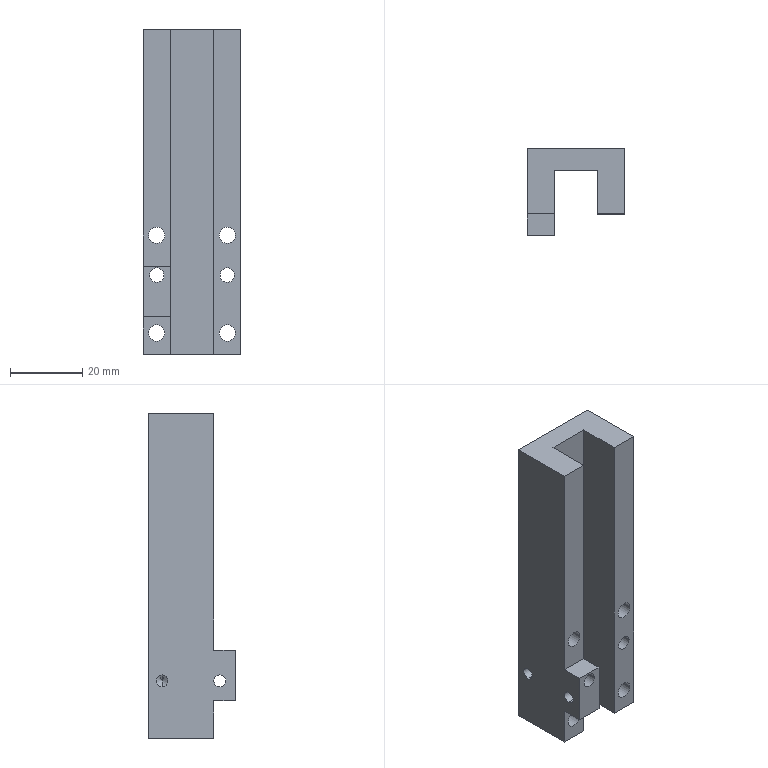Part | NX | features BREP 1 | 1 solid | 32 faces | box 27 x 24 x 90 mm | volume 29584 mm3 | cylinder 16 | plane 14 | cone 2 | commonest cylinder face diameters 4.5 x8 3.3 x4 4 x4
STEP:
#1=CARTESIAN_POINT('',(-774.389,-16.544,14.35));
#2=VERTEX_POINT('',#1);
#3=CARTESIAN_POINT('',(-774.389,-16.544,17.65));
#4=VERTEX_POINT('',#3);
#5=CARTESIAN_POINT('',(-774.389,-16.544,16.));
#6=DIRECTION('',(-1.,0.,0.));
#7=DIRECTION('',(0.,-1.,0.));
#8=AXIS2_PLACEMENT_3D('',#5,#6,#7);
#9=CIRCLE('',#8,1.65);
#10=EDGE_CURVE('',#2,#4,#9,.T.);
#11=ORIENTED_EDGE('',*,*,#10,.F.);
#12=CARTESIAN_POINT('',(-781.889,-16.544,14.35));
#13=VERTEX_POINT('',#12);
#14=CARTESIAN_POINT('',(-781.889,-16.544,14.35));
#15=DIRECTION('',(-1.,0.,0.));
#16=VECTOR('',#15,1000.);
#17=LINE('',#14,#16);
#18=EDGE_CURVE('',#13,#2,#17,.F.);
#19=ORIENTED_EDGE('',*,*,#18,.F.);
#20=CARTESIAN_POINT('',(-781.889,-16.544,17.65));
#21=VERTEX_POINT('',#20);
#22=CARTESIAN_POINT('',(-781.889,-16.544,16.));
#23=DIRECTION('',(-1.,0.,0.));
#24=DIRECTION('',(0.,0.,1.));
#25=AXIS2_PLACEMENT_3D('',#22,#23,#24);
#26=CIRCLE('',#25,1.65);
#27=EDGE_CURVE('',#13,#21,#26,.T.);
#28=ORIENTED_EDGE('',*,*,#27,.T.);
#29=CARTESIAN_POINT('',(-781.889,-16.544,17.65));
#30=DIRECTION('',(-1.,0.,0.));
#31=VECTOR('',#30,1000.);
#32=LINE('',#29,#31);
#33=EDGE_CURVE('',#21,#4,#32,.F.);
#34=ORIENTED_EDGE('',*,*,#33,.T.);
#35=EDGE_LOOP('',(#11,#19,#28,#34));
#36=FACE_BOUND('',#35,.T.);
#37=CARTESIAN_POINT('',(-781.889,-16.544,16.));
#38=DIRECTION('',(-1.,0.,0.));
#39=DIRECTION('',(0.,0.,1.));
#40=AXIS2_PLACEMENT_3D('',#37,#38,#39);
#41=CYLINDRICAL_SURFACE('',#40,1.65);
#42=ADVANCED_FACE('',(#36),#41,.F.);
#43=CARTESIAN_POINT('',(-771.789,-0.5442,14.35));
#44=VERTEX_POINT('',#43);
#45=CARTESIAN_POINT('',(-771.789,-0.5442,17.65));
#46=VERTEX_POINT('',#45);
#47=CARTESIAN_POINT('',(-771.789,-0.5442,16.));
#48=DIRECTION('',(-1.,0.,0.));
#49=DIRECTION('',(0.,0.,1.));
#50=AXIS2_PLACEMENT_3D('',#47,#48,#49);
#51=CIRCLE('',#50,1.65);
#52=EDGE_CURVE('',#44,#46,#51,.T.);
#53=ORIENTED_EDGE('',*,*,#52,.F.);
#54=CARTESIAN_POINT('',(-781.889,-0.5442,14.35));
#55=VERTEX_POINT('',#54);
#56=CARTESIAN_POINT('',(-781.889,-0.5442,14.35));
#57=DIRECTION('',(-1.,0.,0.));
#58=VECTOR('',#57,1000.);
#59=LINE('',#56,#58);
#60=EDGE_CURVE('',#55,#44,#59,.F.);
#61=ORIENTED_EDGE('',*,*,#60,.F.);
#62=CARTESIAN_POINT('',(-781.889,-0.5442,17.65));
#63=VERTEX_POINT('',#62);
#64=CARTESIAN_POINT('',(-781.889,-0.5442,16.));
#65=DIRECTION('',(-1.,0.,0.));
#66=DIRECTION('',(0.,0.,1.));
#67=AXIS2_PLACEMENT_3D('',#64,#65,#66);
#68=CIRCLE('',#67,1.65);
#69=EDGE_CURVE('',#55,#63,#68,.T.);
#70=ORIENTED_EDGE('',*,*,#69,.T.);
#71=CARTESIAN_POINT('',(-781.889,-0.5442,17.65));
#72=DIRECTION('',(-1.,0.,0.));
#73=VECTOR('',#72,1000.);
#74=LINE('',#71,#73);
#75=EDGE_CURVE('',#63,#46,#74,.F.);
#76=ORIENTED_EDGE('',*,*,#75,.T.);
#77=EDGE_LOOP('',(#53,#61,#70,#76));
#78=FACE_BOUND('',#77,.T.);
#79=CARTESIAN_POINT('',(-781.889,-0.5442,16.));
#80=DIRECTION('',(-1.,0.,0.));
#81=DIRECTION('',(0.,0.,1.));
#82=AXIS2_PLACEMENT_3D('',#79,#80,#81);
#83=CYLINDRICAL_SURFACE('',#82,1.65);
#84=ADVANCED_FACE('',(#78),#83,.F.);
#85=CARTESIAN_POINT('',(-770.797,-0.5442,16.));
#86=VERTEX_POINT('',#85);
#87=CARTESIAN_POINT('',(-771.789,-0.5442,17.65));
#88=DIRECTION('',(-0.515,0.,0.8572));
#89=VECTOR('',#88,1000.);
#90=LINE('',#87,#89);
#91=EDGE_CURVE('',#46,#86,#90,.F.);
#92=ORIENTED_EDGE('',*,*,#91,.T.);
#93=CARTESIAN_POINT('',(-771.789,-0.5442,14.35));
#94=DIRECTION('',(-0.515,0.,-0.8572));
#95=VECTOR('',#94,1000.);
#96=LINE('',#93,#95);
#97=EDGE_CURVE('',#44,#86,#96,.F.);
#98=ORIENTED_EDGE('',*,*,#97,.F.);
#99=ORIENTED_EDGE('',*,*,#52,.T.);
#100=EDGE_LOOP('',(#92,#98,#99));
#101=FACE_BOUND('',#100,.T.);
#102=CARTESIAN_POINT('',(-771.789,-0.5442,16.));
#103=DIRECTION('',(-1.,0.,0.));
#104=DIRECTION('',(0.,0.,1.));
#105=AXIS2_PLACEMENT_3D('',#102,#103,#104);
#106=CONICAL_SURFACE('',#105,1.65,1.03);
#107=ADVANCED_FACE('',(#101),#106,.F.);
#108=CARTESIAN_POINT('',(-780.389,3.168,33.));
#109=VERTEX_POINT('',#108);
#110=CARTESIAN_POINT('',(-775.889,3.168,33.));
#111=VERTEX_POINT('',#110);
#112=CARTESIAN_POINT('',(-778.139,3.168,33.));
#113=DIRECTION('',(0.,-1.,0.));
#114=DIRECTION('',(-1.,0.,0.));
#115=AXIS2_PLACEMENT_3D('',#112,#113,#114);
#116=CIRCLE('',#115,2.25);
#117=EDGE_CURVE('',#109,#111,#116,.T.);
#118=ORIENTED_EDGE('',*,*,#117,.F.);
#119=CARTESIAN_POINT('',(-780.389,-14.832,33.));
#120=VERTEX_POINT('',#119);
#121=CARTESIAN_POINT('',(-780.389,3.168,33.));
#122=DIRECTION('',(0.,-1.,0.));
#123=VECTOR('',#122,1000.);
#124=LINE('',#121,#123);
#125=EDGE_CURVE('',#120,#109,#124,.F.);
#126=ORIENTED_EDGE('',*,*,#125,.F.);
#127=CARTESIAN_POINT('',(-775.889,-14.832,33.));
#128=VERTEX_POINT('',#127);
#129=CARTESIAN_POINT('',(-778.139,-14.832,33.));
#130=DIRECTION('',(0.,-1.,0.));
#131=DIRECTION('',(-1.,0.,0.));
#132=AXIS2_PLACEMENT_3D('',#129,#130,#131);
#133=CIRCLE('',#132,2.25);
#134=EDGE_CURVE('',#120,#128,#133,.T.);
#135=ORIENTED_EDGE('',*,*,#134,.T.);
#136=CARTESIAN_POINT('',(-775.889,3.168,33.));
#137=DIRECTION('',(0.,-1.,0.));
#138=VECTOR('',#137,1000.);
#139=LINE('',#136,#138);
#140=EDGE_CURVE('',#128,#111,#139,.F.);
#141=ORIENTED_EDGE('',*,*,#140,.T.);
#142=EDGE_LOOP('',(#118,#126,#135,#141));
#143=FACE_BOUND('',#142,.T.);
#144=CARTESIAN_POINT('',(-778.139,3.168,33.));
#145=DIRECTION('',(0.,-1.,0.));
#146=DIRECTION('',(1.,0.,0.));
#147=AXIS2_PLACEMENT_3D('',#144,#145,#146);
#148=CYLINDRICAL_SURFACE('',#147,2.25);
#149=ADVANCED_FACE('',(#143),#148,.F.);
#150=CARTESIAN_POINT('',(-780.389,3.168,6.));
#151=VERTEX_POINT('',#150);
#152=CARTESIAN_POINT('',(-775.889,3.168,6.));
#153=VERTEX_POINT('',#152);
#154=CARTESIAN_POINT('',(-778.139,3.168,6.));
#155=DIRECTION('',(0.,-1.,0.));
#156=DIRECTION('',(-1.,0.,0.));
#157=AXIS2_PLACEMENT_3D('',#154,#155,#156);
#158=CIRCLE('',#157,2.25);
#159=EDGE_CURVE('',#151,#153,#158,.T.);
#160=ORIENTED_EDGE('',*,*,#159,.F.);
#161=CARTESIAN_POINT('',(-780.389,-14.832,6.));
#162=VERTEX_POINT('',#161);
#163=CARTESIAN_POINT('',(-780.389,3.168,6.));
#164=DIRECTION('',(0.,-1.,0.));
#165=VECTOR('',#164,1000.);
#166=LINE('',#163,#165);
#167=EDGE_CURVE('',#162,#151,#166,.F.);
#168=ORIENTED_EDGE('',*,*,#167,.F.);
#169=CARTESIAN_POINT('',(-775.889,-14.832,6.));
#170=VERTEX_POINT('',#169);
#171=CARTESIAN_POINT('',(-778.139,-14.832,6.));
#172=DIRECTION('',(0.,-1.,0.));
#173=DIRECTION('',(-1.,0.,0.));
#174=AXIS2_PLACEMENT_3D('',#171,#172,#173);
#175=CIRCLE('',#174,2.25);
#176=EDGE_CURVE('',#162,#170,#175,.T.);
#177=ORIENTED_EDGE('',*,*,#176,.T.);
#178=CARTESIAN_POINT('',(-775.889,3.168,6.));
#179=DIRECTION('',(0.,-1.,0.));
#180=VECTOR('',#179,1000.);
#181=LINE('',#178,#180);
#182=EDGE_CURVE('',#170,#153,#181,.F.);
#183=ORIENTED_EDGE('',*,*,#182,.T.);
#184=EDGE_LOOP('',(#160,#168,#177,#183));
#185=FACE_BOUND('',#184,.T.);
#186=CARTESIAN_POINT('',(-778.139,3.168,6.));
#187=DIRECTION('',(0.,-1.,0.));
#188=DIRECTION('',(1.,0.,0.));
#189=AXIS2_PLACEMENT_3D('',#186,#187,#188);
#190=CYLINDRICAL_SURFACE('',#189,2.25);
#191=ADVANCED_FACE('',(#185),#190,.F.);
#192=CARTESIAN_POINT('',(-780.139,3.168,22.));
#193=VERTEX_POINT('',#192);
#194=CARTESIAN_POINT('',(-776.139,3.168,22.));
#195=VERTEX_POINT('',#194);
#196=CARTESIAN_POINT('',(-778.139,3.168,22.));
#197=DIRECTION('',(0.,-1.,0.));
#198=DIRECTION('',(-1.,0.,0.));
#199=AXIS2_PLACEMENT_3D('',#196,#197,#198);
#200=CIRCLE('',#199,2.);
#201=EDGE_CURVE('',#193,#195,#200,.T.);
#202=ORIENTED_EDGE('',*,*,#201,.F.);
#203=CARTESIAN_POINT('',(-780.139,-20.832,22.));
#204=VERTEX_POINT('',#203);
#205=CARTESIAN_POINT('',(-780.139,3.168,22.));
#206=DIRECTION('',(0.,-1.,0.));
#207=VECTOR('',#206,1000.);
#208=LINE('',#205,#207);
#209=EDGE_CURVE('',#204,#193,#208,.F.);
#210=ORIENTED_EDGE('',*,*,#209,.F.);
#211=CARTESIAN_POINT('',(-776.139,-20.832,22.));
#212=VERTEX_POINT('',#211);
#213=CARTESIAN_POINT('',(-778.139,-20.832,22.));
#214=DIRECTION('',(0.,-1.,0.));
#215=DIRECTION('',(1.,0.,0.));
#216=AXIS2_PLACEMENT_3D('',#213,#214,#215);
#217=CIRCLE('',#216,2.);
#218=EDGE_CURVE('',#204,#212,#217,.T.);
#219=ORIENTED_EDGE('',*,*,#218,.T.);
#220=CARTESIAN_POINT('',(-776.139,3.168,22.));
#221=DIRECTION('',(0.,-1.,0.));
#222=VECTOR('',#221,1000.);
#223=LINE('',#220,#222);
#224=EDGE_CURVE('',#212,#195,#223,.F.);
#225=ORIENTED_EDGE('',*,*,#224,.T.);
#226=EDGE_LOOP('',(#202,#210,#219,#225));
#227=FACE_BOUND('',#226,.T.);
#228=CARTESIAN_POINT('',(-778.139,3.168,22.));
#229=DIRECTION('',(0.,-1.,0.));
#230=DIRECTION('',(1.,0.,0.));
#231=AXIS2_PLACEMENT_3D('',#228,#229,#230);
#232=CYLINDRICAL_SURFACE('',#231,2.);
#233=ADVANCED_FACE('',(#227),#232,.F.);
#234=CARTESIAN_POINT('',(-760.639,3.168,22.));
#235=VERTEX_POINT('',#234);
#236=CARTESIAN_POINT('',(-756.639,3.168,22.));
#237=VERTEX_POINT('',#236);
#238=CARTESIAN_POINT('',(-758.639,3.168,22.));
#239=DIRECTION('',(0.,-1.,0.));
#240=DIRECTION('',(1.,0.,0.));
#241=AXIS2_PLACEMENT_3D('',#238,#239,#240);
#242=CIRCLE('',#241,2.);
#243=EDGE_CURVE('',#235,#237,#242,.T.);
#244=ORIENTED_EDGE('',*,*,#243,.F.);
#245=CARTESIAN_POINT('',(-760.639,-14.832,22.));
#246=VERTEX_POINT('',#245);
#247=CARTESIAN_POINT('',(-760.639,3.168,22.));
#248=DIRECTION('',(0.,-1.,0.));
#249=VECTOR('',#248,1000.);
#250=LINE('',#247,#249);
#251=EDGE_CURVE('',#246,#235,#250,.F.);
#252=ORIENTED_EDGE('',*,*,#251,.F.);
#253=CARTESIAN_POINT('',(-756.639,-14.832,22.));
#254=VERTEX_POINT('',#253);
#255=CARTESIAN_POINT('',(-758.639,-14.832,22.));
#256=DIRECTION('',(0.,-1.,0.));
#257=DIRECTION('',(1.,0.,0.));
#258=AXIS2_PLACEMENT_3D('',#255,#256,#257);
#259=CIRCLE('',#258,2.);
#260=EDGE_CURVE('',#246,#254,#259,.T.);
#261=ORIENTED_EDGE('',*,*,#260,.T.);
#262=CARTESIAN_POINT('',(-756.639,3.168,22.));
#263=DIRECTION('',(0.,-1.,0.));
#264=VECTOR('',#263,1000.);
#265=LINE('',#262,#264);
#266=EDGE_CURVE('',#254,#237,#265,.F.);
#267=ORIENTED_EDGE('',*,*,#266,.T.);
#268=EDGE_LOOP('',(#244,#252,#261,#267));
#269=FACE_BOUND('',#268,.T.);
#270=CARTESIAN_POINT('',(-758.639,3.168,22.));
#271=DIRECTION('',(0.,-1.,0.));
#272=DIRECTION('',(1.,0.,0.));
#273=AXIS2_PLACEMENT_3D('',#270,#271,#272);
#274=CYLINDRICAL_SURFACE('',#273,2.);
#275=ADVANCED_FACE('',(#269),#274,.F.);
#276=CARTESIAN_POINT('',(-760.889,3.168,6.));
#277=VERTEX_POINT('',#276);
#278=CARTESIAN_POINT('',(-756.389,3.168,6.));
#279=VERTEX_POINT('',#278);
#280=CARTESIAN_POINT('',(-758.639,3.168,6.));
#281=DIRECTION('',(0.,-1.,0.));
#282=DIRECTION('',(1.,0.,0.));
#283=AXIS2_PLACEMENT_3D('',#280,#281,#282);
#284=CIRCLE('',#283,2.25);
#285=EDGE_CURVE('',#277,#279,#284,.T.);
#286=ORIENTED_EDGE('',*,*,#285,.F.);
#287=CARTESIAN_POINT('',(-760.889,-14.832,6.));
#288=VERTEX_POINT('',#287);
#289=CARTESIAN_POINT('',(-760.889,3.168,6.));
#290=DIRECTION('',(0.,-1.,0.));
#291=VECTOR('',#290,1000.);
#292=LINE('',#289,#291);
#293=EDGE_CURVE('',#288,#277,#292,.F.);
#294=ORIENTED_EDGE('',*,*,#293,.F.);
#295=CARTESIAN_POINT('',(-756.389,-14.832,6.));
#296=VERTEX_POINT('',#295);
#297=CARTESIAN_POINT('',(-758.639,-14.832,6.));
#298=DIRECTION('',(0.,-1.,0.));
#299=DIRECTION('',(1.,0.,0.));
#300=AXIS2_PLACEMENT_3D('',#297,#298,#299);
#301=CIRCLE('',#300,2.25);
#302=EDGE_CURVE('',#288,#296,#301,.T.);
#303=ORIENTED_EDGE('',*,*,#302,.T.);
#304=CARTESIAN_POINT('',(-756.389,3.168,6.));
#305=DIRECTION('',(0.,-1.,0.));
#306=VECTOR('',#305,1000.);
#307=LINE('',#304,#306);
#308=EDGE_CURVE('',#296,#279,#307,.F.);
#309=ORIENTED_EDGE('',*,*,#308,.T.);
#310=EDGE_LOOP('',(#286,#294,#303,#309));
#311=FACE_BOUND('',#310,.T.);
#312=CARTESIAN_POINT('',(-758.639,3.168,6.));
#313=DIRECTION('',(0.,-1.,0.));
#314=DIRECTION('',(1.,0.,0.));
#315=AXIS2_PLACEMENT_3D('',#312,#313,#314);
#316=CYLINDRICAL_SURFACE('',#315,2.25);
#317=ADVANCED_FACE('',(#311),#316,.F.);
#318=CARTESIAN_POINT('',(-760.889,3.168,33.));
#319=VERTEX_POINT('',#318);
#320=CARTESIAN_POINT('',(-756.389,3.168,33.));
#321=VERTEX_POINT('',#320);
#322=CARTESIAN_POINT('',(-758.639,3.168,33.));
#323=DIRECTION('',(0.,-1.,0.));
#324=DIRECTION('',(1.,0.,0.));
#325=AXIS2_PLACEMENT_3D('',#322,#323,#324);
#326=CIRCLE('',#325,2.25);
#327=EDGE_CURVE('',#319,#321,#326,.T.);
#328=ORIENTED_EDGE('',*,*,#327,.F.);
#329=CARTESIAN_POINT('',(-760.889,-14.832,33.));
#330=VERTEX_POINT('',#329);
#331=CARTESIAN_POINT('',(-760.889,3.168,33.));
#332=DIRECTION('',(0.,-1.,0.));
#333=VECTOR('',#332,1000.);
#334=LINE('',#331,#333);
#335=EDGE_CURVE('',#330,#319,#334,.F.);
#336=ORIENTED_EDGE('',*,*,#335,.F.);
#337=CARTESIAN_POINT('',(-756.389,-14.832,33.));
#338=VERTEX_POINT('',#337);
#339=CARTESIAN_POINT('',(-758.639,-14.832,33.));
#340=DIRECTION('',(0.,-1.,0.));
#341=DIRECTION('',(1.,0.,0.));
#342=AXIS2_PLACEMENT_3D('',#339,#340,#341);
#343=CIRCLE('',#342,2.25);
#344=EDGE_CURVE('',#330,#338,#343,.T.);
#345=ORIENTED_EDGE('',*,*,#344,.T.);
#346=CARTESIAN_POINT('',(-756.389,3.168,33.));
#347=DIRECTION('',(0.,-1.,0.));
#348=VECTOR('',#347,1000.);
#349=LINE('',#346,#348);
#350=EDGE_CURVE('',#338,#321,#349,.F.);
#351=ORIENTED_EDGE('',*,*,#350,.T.);
#352=EDGE_LOOP('',(#328,#336,#345,#351));
#353=FACE_BOUND('',#352,.T.);
#354=CARTESIAN_POINT('',(-758.639,3.168,33.));
#355=DIRECTION('',(0.,-1.,0.));
#356=DIRECTION('',(1.,0.,0.));
#357=AXIS2_PLACEMENT_3D('',#354,#355,#356);
#358=CYLINDRICAL_SURFACE('',#357,2.25);
#359=ADVANCED_FACE('',(#353),#358,.F.);
#360=CARTESIAN_POINT('',(-774.389,-14.832,24.5));
#361=VERTEX_POINT('',#360);
#362=CARTESIAN_POINT('',(-781.889,-14.832,24.5));
#363=VERTEX_POINT('',#362);
#364=CARTESIAN_POINT('',(-774.389,-14.832,24.5));
#365=DIRECTION('',(-1.,0.,0.));
#366=VECTOR('',#365,1000.);
#367=LINE('',#364,#366);
#368=EDGE_CURVE('',#361,#363,#367,.T.);
#369=ORIENTED_EDGE('',*,*,#368,.F.);
#370=CARTESIAN_POINT('',(-774.389,-14.832,90.));
#371=VERTEX_POINT('',#370);
#372=CARTESIAN_POINT('',(-774.389,-14.832,0.));
#373=DIRECTION('',(0.,0.,1.));
#374=VECTOR('',#373,1000.);
#375=LINE('',#372,#374);
#376=EDGE_CURVE('',#361,#371,#375,.T.);
#377=ORIENTED_EDGE('',*,*,#376,.T.);
#378=CARTESIAN_POINT('',(-781.889,-14.832,90.));
#379=VERTEX_POINT('',#378);
#380=CARTESIAN_POINT('',(-754.889,-14.832,90.));
#381=DIRECTION('',(1.,0.,0.));
#382=VECTOR('',#381,1000.);
#383=LINE('',#380,#382);
#384=EDGE_CURVE('',#379,#371,#383,.T.);
#385=ORIENTED_EDGE('',*,*,#384,.F.);
#386=CARTESIAN_POINT('',(-781.889,-14.832,90.));
#387=DIRECTION('',(0.,0.,-1.));
#388=VECTOR('',#387,1000.);
#389=LINE('',#386,#388);
#390=EDGE_CURVE('',#379,#363,#389,.T.);
#391=ORIENTED_EDGE('',*,*,#390,.T.);
#392=EDGE_LOOP('',(#369,#377,#385,#391));
#393=FACE_BOUND('',#392,.T.);
#394=CARTESIAN_POINT('',(-778.139,-14.832,33.));
#395=DIRECTION('',(0.,-1.,0.));
#396=DIRECTION('',(-1.,0.,0.));
#397=AXIS2_PLACEMENT_3D('',#394,#395,#396);
#398=CIRCLE('',#397,2.25);
#399=EDGE_CURVE('',#128,#120,#398,.T.);
#400=ORIENTED_EDGE('',*,*,#399,.F.);
#401=ORIENTED_EDGE('',*,*,#134,.F.);
#402=EDGE_LOOP('',(#400,#401));
#403=FACE_BOUND('',#402,.T.);
#404=CARTESIAN_POINT('',(-754.889,-14.832,90.));
#405=DIRECTION('',(0.,1.,0.));
#406=DIRECTION('',(1.,0.,0.));
#407=AXIS2_PLACEMENT_3D('',#404,#405,#406);
#408=PLANE('',#407);
#409=ADVANCED_FACE('',(#393,#403),#408,.F.);
#410=CARTESIAN_POINT('',(-781.889,-14.832,10.5));
#411=VERTEX_POINT('',#410);
#412=CARTESIAN_POINT('',(-774.389,-14.832,10.5));
#413=VERTEX_POINT('',#412);
#414=CARTESIAN_POINT('',(-774.389,-14.832,10.5));
#415=DIRECTION('',(1.,0.,0.));
#416=VECTOR('',#415,1000.);
#417=LINE('',#414,#416);
#418=EDGE_CURVE('',#411,#413,#417,.T.);
#419=ORIENTED_EDGE('',*,*,#418,.F.);
#420=CARTESIAN_POINT('',(-781.889,-14.832,0.));
#421=VERTEX_POINT('',#420);
#422=CARTESIAN_POINT('',(-781.889,-14.832,90.));
#423=DIRECTION('',(0.,0.,-1.));
#424=VECTOR('',#423,1000.);
#425=LINE('',#422,#424);
#426=EDGE_CURVE('',#411,#421,#425,.T.);
#427=ORIENTED_EDGE('',*,*,#426,.T.);
#428=CARTESIAN_POINT('',(-774.389,-14.832,0.));
#429=VERTEX_POINT('',#428);
#430=CARTESIAN_POINT('',(-754.889,-14.832,0.));
#431=DIRECTION('',(1.,0.,0.));
#432=VECTOR('',#431,1000.);
#433=LINE('',#430,#432);
#434=EDGE_CURVE('',#421,#429,#433,.T.);
#435=ORIENTED_EDGE('',*,*,#434,.T.);
#436=CARTESIAN_POINT('',(-774.389,-14.832,0.));
#437=DIRECTION('',(0.,0.,1.));
#438=VECTOR('',#437,1000.);
#439=LINE('',#436,#438);
#440=EDGE_CURVE('',#429,#413,#439,.T.);
#441=ORIENTED_EDGE('',*,*,#440,.T.);
#442=EDGE_LOOP('',(#419,#427,#435,#441));
#443=FACE_BOUND('',#442,.T.);
#444=CARTESIAN_POINT('',(-778.139,-14.832,6.));
#445=DIRECTION('',(0.,-1.,0.));
#446=DIRECTION('',(-1.,0.,0.));
#447=AXIS2_PLACEMENT_3D('',#444,#445,#446);
#448=CIRCLE('',#447,2.25);
#449=EDGE_CURVE('',#170,#162,#448,.T.);
#450=ORIENTED_EDGE('',*,*,#449,.F.);
#451=ORIENTED_EDGE('',*,*,#176,.F.);
#452=EDGE_LOOP('',(#450,#451));
#453=FACE_BOUND('',#452,.T.);
#454=CARTESIAN_POINT('',(-754.889,-14.832,90.));
#455=DIRECTION('',(0.,1.,0.));
#456=DIRECTION('',(1.,0.,0.));
#457=AXIS2_PLACEMENT_3D('',#454,#455,#456);
#458=PLANE('',#457);
#459=ADVANCED_FACE('',(#443,#453),#458,.F.);
#460=CARTESIAN_POINT('',(-762.389,-14.832,90.));
#461=VERTEX_POINT('',#460);
#462=CARTESIAN_POINT('',(-754.889,-14.832,90.));
#463=VERTEX_POINT('',#462);
#464=CARTESIAN_POINT('',(-754.889,-14.832,90.));
#465=DIRECTION('',(1.,0.,0.));
#466=VECTOR('',#465,1000.);
#467=LINE('',#464,#466);
#468=EDGE_CURVE('',#461,#463,#467,.T.);
#469=ORIENTED_EDGE('',*,*,#468,.F.);
#470=CARTESIAN_POINT('',(-762.389,-14.832,0.));
#471=VERTEX_POINT('',#470);
#472=CARTESIAN_POINT('',(-762.389,-14.832,0.));
#473=DIRECTION('',(0.,0.,1.));
#474=VECTOR('',#473,1000.);
#475=LINE('',#472,#474);
#476=EDGE_CURVE('',#471,#461,#475,.T.);
#477=ORIENTED_EDGE('',*,*,#476,.F.);
#478=CARTESIAN_POINT('',(-754.889,-14.832,0.));
#479=VERTEX_POINT('',#478);
#480=CARTESIAN_POINT('',(-754.889,-14.832,0.));
#481=DIRECTION('',(1.,0.,0.));
#482=VECTOR('',#481,1000.);
#483=LINE('',#480,#482);
#484=EDGE_CURVE('',#471,#479,#483,.T.);
#485=ORIENTED_EDGE('',*,*,#484,.T.);
#486=CARTESIAN_POINT('',(-754.889,-14.832,90.));
#487=DIRECTION('',(0.,0.,-1.));
#488=VECTOR('',#487,1000.);
#489=LINE('',#486,#488);
#490=EDGE_CURVE('',#463,#479,#489,.T.);
#491=ORIENTED_EDGE('',*,*,#490,.F.);
#492=EDGE_LOOP('',(#469,#477,#485,#491));
#493=FACE_BOUND('',#492,.T.);
#494=CARTESIAN_POINT('',(-758.639,-14.832,22.));
#495=DIRECTION('',(0.,-1.,0.));
#496=DIRECTION('',(1.,0.,0.));
#497=AXIS2_PLACEMENT_3D('',#494,#495,#496);
#498=CIRCLE('',#497,2.);
#499=EDGE_CURVE('',#254,#246,#498,.T.);
#500=ORIENTED_EDGE('',*,*,#499,.F.);
#501=ORIENTED_EDGE('',*,*,#260,.F.);
#502=EDGE_LOOP('',(#500,#501));
#503=FACE_BOUND('',#502,.T.);
#504=CARTESIAN_POINT('',(-758.639,-14.832,6.));
#505=DIRECTION('',(0.,-1.,0.));
#506=DIRECTION('',(1.,0.,0.));
#507=AXIS2_PLACEMENT_3D('',#504,#505,#506);
#508=CIRCLE('',#507,2.25);
#509=EDGE_CURVE('',#296,#288,#508,.T.);
#510=ORIENTED_EDGE('',*,*,#509,.F.);
#511=ORIENTED_EDGE('',*,*,#302,.F.);
#512=EDGE_LOOP('',(#510,#511));
#513=FACE_BOUND('',#512,.T.);
#514=CARTESIAN_POINT('',(-758.639,-14.832,33.));
#515=DIRECTION('',(0.,-1.,0.));
#516=DIRECTION('',(1.,0.,0.));
#517=AXIS2_PLACEMENT_3D('',#514,#515,#516);
#518=CIRCLE('',#517,2.25);
#519=EDGE_CURVE('',#338,#330,#518,.T.);
#520=ORIENTED_EDGE('',*,*,#519,.F.);
#521=ORIENTED_EDGE('',*,*,#344,.F.);
#522=EDGE_LOOP('',(#520,#521));
#523=FACE_BOUND('',#522,.T.);
#524=CARTESIAN_POINT('',(-754.889,-14.832,90.));
#525=DIRECTION('',(0.,1.,0.));
#526=DIRECTION('',(1.,0.,0.));
#527=AXIS2_PLACEMENT_3D('',#524,#525,#526);
#528=PLANE('',#527);
#529=ADVANCED_FACE('',(#493,#503,#513,#523),#528,.F.);
#530=CARTESIAN_POINT('',(-754.889,3.168,0.));
#531=VERTEX_POINT('',#530);
#532=CARTESIAN_POINT('',(-754.889,-14.832,0.));
#533=DIRECTION('',(0.,1.,0.));
#534=VECTOR('',#533,1000.);
#535=LINE('',#532,#534);
#536=EDGE_CURVE('',#479,#531,#535,.T.);
#537=ORIENTED_EDGE('',*,*,#536,.T.);
#538=CARTESIAN_POINT('',(-754.889,3.168,90.));
#539=VERTEX_POINT('',#538);
#540=CARTESIAN_POINT('',(-754.889,3.168,90.));
#541=DIRECTION('',(0.,0.,-1.));
#542=VECTOR('',#541,1000.);
#543=LINE('',#540,#542);
#544=EDGE_CURVE('',#539,#531,#543,.T.);
#545=ORIENTED_EDGE('',*,*,#544,.F.);
#546=CARTESIAN_POINT('',(-754.889,-14.832,90.));
#547=DIRECTION('',(0.,1.,0.));
#548=VECTOR('',#547,1000.);
#549=LINE('',#546,#548);
#550=EDGE_CURVE('',#463,#539,#549,.T.);
#551=ORIENTED_EDGE('',*,*,#550,.F.);
#552=ORIENTED_EDGE('',*,*,#490,.T.);
#553=EDGE_LOOP('',(#537,#545,#551,#552));
#554=FACE_BOUND('',#553,.T.);
#555=CARTESIAN_POINT('',(-754.889,-14.832,90.));
#556=DIRECTION('',(-1.,0.,0.));
#557=DIRECTION('',(0.,0.,1.));
#558=AXIS2_PLACEMENT_3D('',#555,#556,#557);
#559=PLANE('',#558);
#560=ADVANCED_FACE('',(#554),#559,.F.);
#561=CARTESIAN_POINT('',(-781.889,3.168,0.));
#562=VERTEX_POINT('',#561);
#563=CARTESIAN_POINT('',(-754.889,3.168,0.));
#564=DIRECTION('',(-1.,0.,0.));
#565=VECTOR('',#564,1000.);
#566=LINE('',#563,#565);
#567=EDGE_CURVE('',#531,#562,#566,.T.);
#568=ORIENTED_EDGE('',*,*,#567,.T.);
#569=CARTESIAN_POINT('',(-781.889,3.168,90.));
#570=VERTEX_POINT('',#569);
#571=CARTESIAN_POINT('',(-781.889,3.168,90.));
#572=DIRECTION('',(0.,0.,-1.));
#573=VECTOR('',#572,1000.);
#574=LINE('',#571,#573);
#575=EDGE_CURVE('',#570,#562,#574,.T.);
#576=ORIENTED_EDGE('',*,*,#575,.F.);
#577=CARTESIAN_POINT('',(-754.889,3.168,90.));
#578=DIRECTION('',(-1.,0.,0.));
#579=VECTOR('',#578,1000.);
#580=LINE('',#577,#579);
#581=EDGE_CURVE('',#539,#570,#580,.T.);
#582=ORIENTED_EDGE('',*,*,#581,.F.);
#583=ORIENTED_EDGE('',*,*,#544,.T.);
#584=EDGE_LOOP('',(#568,#576,#582,#583));
#585=FACE_BOUND('',#584,.T.);
#586=CARTESIAN_POINT('',(-778.139,3.168,33.));
#587=DIRECTION('',(0.,-1.,0.));
#588=DIRECTION('',(-1.,0.,0.));
#589=AXIS2_PLACEMENT_3D('',#586,#587,#588);
#590=CIRCLE('',#589,2.25);
#591=EDGE_CURVE('',#111,#109,#590,.T.);
#592=ORIENTED_EDGE('',*,*,#591,.T.);
#593=ORIENTED_EDGE('',*,*,#117,.T.);
#594=EDGE_LOOP('',(#592,#593));
#595=FACE_BOUND('',#594,.T.);
#596=CARTESIAN_POINT('',(-778.139,3.168,6.));
#597=DIRECTION('',(0.,-1.,0.));
#598=DIRECTION('',(-1.,0.,0.));
#599=AXIS2_PLACEMENT_3D('',#596,#597,#598);
#600=CIRCLE('',#599,2.25);
#601=EDGE_CURVE('',#153,#151,#600,.T.);
#602=ORIENTED_EDGE('',*,*,#601,.T.);
#603=ORIENTED_EDGE('',*,*,#159,.T.);
#604=EDGE_LOOP('',(#602,#603));
#605=FACE_BOUND('',#604,.T.);
#606=CARTESIAN_POINT('',(-778.139,3.168,22.));
#607=DIRECTION('',(0.,-1.,0.));
#608=DIRECTION('',(-1.,0.,0.));
#609=AXIS2_PLACEMENT_3D('',#606,#607,#608);
#610=CIRCLE('',#609,2.);
#611=EDGE_CURVE('',#195,#193,#610,.T.);
#612=ORIENTED_EDGE('',*,*,#611,.T.);
#613=ORIENTED_EDGE('',*,*,#201,.T.);
#614=EDGE_LOOP('',(#612,#613));
#615=FACE_BOUND('',#614,.T.);
#616=CARTESIAN_POINT('',(-758.639,3.168,22.));
#617=DIRECTION('',(0.,-1.,0.));
#618=DIRECTION('',(1.,0.,0.));
#619=AXIS2_PLACEMENT_3D('',#616,#617,#618);
#620=CIRCLE('',#619,2.);
#621=EDGE_CURVE('',#237,#235,#620,.T.);
#622=ORIENTED_EDGE('',*,*,#621,.T.);
#623=ORIENTED_EDGE('',*,*,#243,.T.);
#624=EDGE_LOOP('',(#622,#623));
#625=FACE_BOUND('',#624,.T.);
#626=CARTESIAN_POINT('',(-758.639,3.168,6.));
#627=DIRECTION('',(0.,-1.,0.));
#628=DIRECTION('',(1.,0.,0.));
#629=AXIS2_PLACEMENT_3D('',#626,#627,#628);
#630=CIRCLE('',#629,2.25);
#631=EDGE_CURVE('',#279,#277,#630,.T.);
#632=ORIENTED_EDGE('',*,*,#631,.T.);
#633=ORIENTED_EDGE('',*,*,#285,.T.);
#634=EDGE_LOOP('',(#632,#633));
#635=FACE_BOUND('',#634,.T.);
#636=CARTESIAN_POINT('',(-758.639,3.168,33.));
#637=DIRECTION('',(0.,-1.,0.));
#638=DIRECTION('',(1.,0.,0.));
#639=AXIS2_PLACEMENT_3D('',#636,#637,#638);
#640=CIRCLE('',#639,2.25);
#641=EDGE_CURVE('',#321,#319,#640,.T.);
#642=ORIENTED_EDGE('',*,*,#641,.T.);
#643=ORIENTED_EDGE('',*,*,#327,.T.);
#644=EDGE_LOOP('',(#642,#643));
#645=FACE_BOUND('',#644,.T.);
#646=CARTESIAN_POINT('',(-754.889,3.168,90.));
#647=DIRECTION('',(0.,-1.,0.));
#648=DIRECTION('',(0.,0.,-1.));
#649=AXIS2_PLACEMENT_3D('',#646,#647,#648);
#650=PLANE('',#649);
#651=ADVANCED_FACE('',(#585,#595,#605,#615,#625,#635,#645),#650,.F.);
#652=CARTESIAN_POINT('',(-781.889,-14.832,0.));
#653=DIRECTION('',(0.,-1.,0.));
#654=VECTOR('',#653,1000.);
#655=LINE('',#652,#654);
#656=EDGE_CURVE('',#562,#421,#655,.T.);
#657=ORIENTED_EDGE('',*,*,#656,.T.);
#658=ORIENTED_EDGE('',*,*,#426,.F.);
#659=CARTESIAN_POINT('',(-781.889,-20.832,10.5));
#660=VERTEX_POINT('',#659);
#661=CARTESIAN_POINT('',(-781.889,-20.832,10.5));
#662=DIRECTION('',(0.,1.,0.));
#663=VECTOR('',#662,1000.);
#664=LINE('',#661,#663);
#665=EDGE_CURVE('',#660,#411,#664,.T.);
#666=ORIENTED_EDGE('',*,*,#665,.F.);
#667=CARTESIAN_POINT('',(-781.889,-20.832,24.5));
#668=VERTEX_POINT('',#667);
#669=CARTESIAN_POINT('',(-781.889,-20.832,24.5));
#670=DIRECTION('',(0.,0.,-1.));
#671=VECTOR('',#670,1000.);
#672=LINE('',#669,#671);
#673=EDGE_CURVE('',#668,#660,#672,.T.);
#674=ORIENTED_EDGE('',*,*,#673,.F.);
#675=CARTESIAN_POINT('',(-781.889,-20.832,24.5));
#676=DIRECTION('',(0.,1.,0.));
#677=VECTOR('',#676,1000.);
#678=LINE('',#675,#677);
#679=EDGE_CURVE('',#668,#363,#678,.T.);
#680=ORIENTED_EDGE('',*,*,#679,.T.);
#681=ORIENTED_EDGE('',*,*,#390,.F.);
#682=CARTESIAN_POINT('',(-781.889,-14.832,90.));
#683=DIRECTION('',(0.,-1.,0.));
#684=VECTOR('',#683,1000.);
#685=LINE('',#682,#684);
#686=EDGE_CURVE('',#570,#379,#685,.T.);
#687=ORIENTED_EDGE('',*,*,#686,.F.);
#688=ORIENTED_EDGE('',*,*,#575,.T.);
#689=EDGE_LOOP('',(#657,#658,#666,#674,#680,#681,#687,#688));
#690=FACE_BOUND('',#689,.T.);
#691=CARTESIAN_POINT('',(-781.889,-16.544,16.));
#692=DIRECTION('',(-1.,0.,0.));
#693=DIRECTION('',(0.,0.,1.));
#694=AXIS2_PLACEMENT_3D('',#691,#692,#693);
#695=CIRCLE('',#694,1.65);
#696=EDGE_CURVE('',#21,#13,#695,.T.);
#697=ORIENTED_EDGE('',*,*,#696,.F.);
#698=ORIENTED_EDGE('',*,*,#27,.F.);
#699=EDGE_LOOP('',(#697,#698));
#700=FACE_BOUND('',#699,.T.);
#701=CARTESIAN_POINT('',(-781.889,-0.5442,16.));
#702=DIRECTION('',(-1.,0.,0.));
#703=DIRECTION('',(0.,0.,1.));
#704=AXIS2_PLACEMENT_3D('',#701,#702,#703);
#705=CIRCLE('',#704,1.65);
#706=EDGE_CURVE('',#63,#55,#705,.T.);
#707=ORIENTED_EDGE('',*,*,#706,.F.);
#708=ORIENTED_EDGE('',*,*,#69,.F.);
#709=EDGE_LOOP('',(#707,#708));
#710=FACE_BOUND('',#709,.T.);
#711=CARTESIAN_POINT('',(-781.889,-14.832,90.));
#712=DIRECTION('',(1.,0.,0.));
#713=DIRECTION('',(0.,1.,0.));
#714=AXIS2_PLACEMENT_3D('',#711,#712,#713);
#715=PLANE('',#714);
#716=ADVANCED_FACE('',(#690,#700,#710),#715,.F.);
#717=CARTESIAN_POINT('',(-762.389,-2.832,90.));
#718=VERTEX_POINT('',#717);
#719=CARTESIAN_POINT('',(-762.389,-14.832,90.));
#720=DIRECTION('',(0.,1.,0.));
#721=VECTOR('',#720,1000.);
#722=LINE('',#719,#721);
#723=EDGE_CURVE('',#461,#718,#722,.T.);
#724=ORIENTED_EDGE('',*,*,#723,.F.);
#725=ORIENTED_EDGE('',*,*,#468,.T.);
#726=ORIENTED_EDGE('',*,*,#550,.T.);
#727=ORIENTED_EDGE('',*,*,#581,.T.);
#728=ORIENTED_EDGE('',*,*,#686,.T.);
#729=ORIENTED_EDGE('',*,*,#384,.T.);
#730=CARTESIAN_POINT('',(-774.389,-2.832,90.));
#731=VERTEX_POINT('',#730);
#732=CARTESIAN_POINT('',(-774.389,-14.832,90.));
#733=DIRECTION('',(0.,-1.,0.));
#734=VECTOR('',#733,1000.);
#735=LINE('',#732,#734);
#736=EDGE_CURVE('',#731,#371,#735,.T.);
#737=ORIENTED_EDGE('',*,*,#736,.F.);
#738=CARTESIAN_POINT('',(-762.389,-2.832,90.));
#739=DIRECTION('',(-1.,0.,0.));
#740=VECTOR('',#739,1000.);
#741=LINE('',#738,#740);
#742=EDGE_CURVE('',#718,#731,#741,.T.);
#743=ORIENTED_EDGE('',*,*,#742,.F.);
#744=EDGE_LOOP('',(#724,#725,#726,#727,#728,#729,#737,#743));
#745=FACE_BOUND('',#744,.T.);
#746=CARTESIAN_POINT('',(-754.889,3.168,90.));
#747=DIRECTION('',(0.,0.,1.));
#748=DIRECTION('',(1.,0.,0.));
#749=AXIS2_PLACEMENT_3D('',#746,#747,#748);
#750=PLANE('',#749);
#751=ADVANCED_FACE('',(#745),#750,.T.);
#752=ORIENTED_EDGE('',*,*,#484,.F.);
#753=CARTESIAN_POINT('',(-762.389,-2.832,0.));
#754=VERTEX_POINT('',#753);
#755=CARTESIAN_POINT('',(-762.389,-14.832,0.));
#756=DIRECTION('',(0.,1.,0.));
#757=VECTOR('',#756,1000.);
#758=LINE('',#755,#757);
#759=EDGE_CURVE('',#471,#754,#758,.T.);
#760=ORIENTED_EDGE('',*,*,#759,.T.);
#761=CARTESIAN_POINT('',(-774.389,-2.832,0.));
#762=VERTEX_POINT('',#761);
#763=CARTESIAN_POINT('',(-762.389,-2.832,0.));
#764=DIRECTION('',(-1.,0.,0.));
#765=VECTOR('',#764,1000.);
#766=LINE('',#763,#765);
#767=EDGE_CURVE('',#754,#762,#766,.T.);
#768=ORIENTED_EDGE('',*,*,#767,.T.);
#769=CARTESIAN_POINT('',(-774.389,-14.832,0.));
#770=DIRECTION('',(0.,-1.,0.));
#771=VECTOR('',#770,1000.);
#772=LINE('',#769,#771);
#773=EDGE_CURVE('',#762,#429,#772,.T.);
#774=ORIENTED_EDGE('',*,*,#773,.T.);
#775=ORIENTED_EDGE('',*,*,#434,.F.);
#776=ORIENTED_EDGE('',*,*,#656,.F.);
#777=ORIENTED_EDGE('',*,*,#567,.F.);
#778=ORIENTED_EDGE('',*,*,#536,.F.);
#779=EDGE_LOOP('',(#752,#760,#768,#774,#775,#776,#777,#778));
#780=FACE_BOUND('',#779,.T.);
#781=CARTESIAN_POINT('',(-754.889,3.168,0.));
#782=DIRECTION('',(0.,0.,1.));
#783=DIRECTION('',(1.,0.,0.));
#784=AXIS2_PLACEMENT_3D('',#781,#782,#783);
#785=PLANE('',#784);
#786=ADVANCED_FACE('',(#780),#785,.F.);
#787=ORIENTED_EDGE('',*,*,#723,.T.);
#788=CARTESIAN_POINT('',(-762.389,-2.832,0.));
#789=DIRECTION('',(0.,0.,1.));
#790=VECTOR('',#789,1000.);
#791=LINE('',#788,#790);
#792=EDGE_CURVE('',#754,#718,#791,.T.);
#793=ORIENTED_EDGE('',*,*,#792,.F.);
#794=ORIENTED_EDGE('',*,*,#759,.F.);
#795=ORIENTED_EDGE('',*,*,#476,.T.);
#796=EDGE_LOOP('',(#787,#793,#794,#795));
#797=FACE_BOUND('',#796,.T.);
#798=CARTESIAN_POINT('',(-762.389,-14.832,0.));
#799=DIRECTION('',(1.,0.,0.));
#800=DIRECTION('',(0.,1.,0.));
#801=AXIS2_PLACEMENT_3D('',#798,#799,#800);
#802=PLANE('',#801);
#803=ADVANCED_FACE('',(#797),#802,.F.);
#804=ORIENTED_EDGE('',*,*,#736,.T.);
#805=ORIENTED_EDGE('',*,*,#376,.F.);
#806=CARTESIAN_POINT('',(-774.389,-20.832,24.5));
#807=VERTEX_POINT('',#806);
#808=CARTESIAN_POINT('',(-774.389,-20.832,24.5));
#809=DIRECTION('',(0.,1.,0.));
#810=VECTOR('',#809,1000.);
#811=LINE('',#808,#810);
#812=EDGE_CURVE('',#807,#361,#811,.T.);
#813=ORIENTED_EDGE('',*,*,#812,.F.);
#814=CARTESIAN_POINT('',(-774.389,-20.832,10.5));
#815=VERTEX_POINT('',#814);
#816=CARTESIAN_POINT('',(-774.389,-20.832,24.5));
#817=DIRECTION('',(0.,0.,1.));
#818=VECTOR('',#817,1000.);
#819=LINE('',#816,#818);
#820=EDGE_CURVE('',#815,#807,#819,.T.);
#821=ORIENTED_EDGE('',*,*,#820,.F.);
#822=CARTESIAN_POINT('',(-774.389,-20.832,10.5));
#823=DIRECTION('',(0.,1.,0.));
#824=VECTOR('',#823,1000.);
#825=LINE('',#822,#824);
#826=EDGE_CURVE('',#815,#413,#825,.T.);
#827=ORIENTED_EDGE('',*,*,#826,.T.);
#828=ORIENTED_EDGE('',*,*,#440,.F.);
#829=ORIENTED_EDGE('',*,*,#773,.F.);
#830=CARTESIAN_POINT('',(-774.389,-2.832,0.));
#831=DIRECTION('',(0.,0.,1.));
#832=VECTOR('',#831,1000.);
#833=LINE('',#830,#832);
#834=EDGE_CURVE('',#762,#731,#833,.T.);
#835=ORIENTED_EDGE('',*,*,#834,.T.);
#836=EDGE_LOOP('',(#804,#805,#813,#821,#827,#828,#829,#835));
#837=FACE_BOUND('',#836,.T.);
#838=CARTESIAN_POINT('',(-774.389,-16.544,16.));
#839=DIRECTION('',(-1.,0.,0.));
#840=DIRECTION('',(0.,-1.,0.));
#841=AXIS2_PLACEMENT_3D('',#838,#839,#840);
#842=CIRCLE('',#841,1.65);
#843=EDGE_CURVE('',#4,#2,#842,.T.);
#844=ORIENTED_EDGE('',*,*,#843,.T.);
#845=ORIENTED_EDGE('',*,*,#10,.T.);
#846=EDGE_LOOP('',(#844,#845));
#847=FACE_BOUND('',#846,.T.);
#848=CARTESIAN_POINT('',(-774.389,-14.832,0.));
#849=DIRECTION('',(-1.,0.,0.));
#850=DIRECTION('',(0.,1.,0.));
#851=AXIS2_PLACEMENT_3D('',#848,#849,#850);
#852=PLANE('',#851);
#853=ADVANCED_FACE('',(#837,#847),#852,.F.);
#854=ORIENTED_EDGE('',*,*,#742,.T.);
#855=ORIENTED_EDGE('',*,*,#834,.F.);
#856=ORIENTED_EDGE('',*,*,#767,.F.);
#857=ORIENTED_EDGE('',*,*,#792,.T.);
#858=EDGE_LOOP('',(#854,#855,#856,#857));
#859=FACE_BOUND('',#858,.T.);
#860=CARTESIAN_POINT('',(-762.389,-2.832,0.));
#861=DIRECTION('',(0.,1.,0.));
#862=DIRECTION('',(1.,0.,0.));
#863=AXIS2_PLACEMENT_3D('',#860,#861,#862);
#864=PLANE('',#863);
#865=ADVANCED_FACE('',(#859),#864,.F.);
#866=ORIENTED_EDGE('',*,*,#335,.T.);
#867=ORIENTED_EDGE('',*,*,#641,.F.);
#868=ORIENTED_EDGE('',*,*,#350,.F.);
#869=ORIENTED_EDGE('',*,*,#519,.T.);
#870=EDGE_LOOP('',(#866,#867,#868,#869));
#871=FACE_BOUND('',#870,.T.);
#872=CARTESIAN_POINT('',(-758.639,3.168,33.));
#873=DIRECTION('',(0.,-1.,0.));
#874=DIRECTION('',(1.,0.,0.));
#875=AXIS2_PLACEMENT_3D('',#872,#873,#874);
#876=CYLINDRICAL_SURFACE('',#875,2.25);
#877=ADVANCED_FACE('',(#871),#876,.F.);
#878=ORIENTED_EDGE('',*,*,#293,.T.);
#879=ORIENTED_EDGE('',*,*,#631,.F.);
#880=ORIENTED_EDGE('',*,*,#308,.F.);
#881=ORIENTED_EDGE('',*,*,#509,.T.);
#882=EDGE_LOOP('',(#878,#879,#880,#881));
#883=FACE_BOUND('',#882,.T.);
#884=CARTESIAN_POINT('',(-758.639,3.168,6.));
#885=DIRECTION('',(0.,-1.,0.));
#886=DIRECTION('',(1.,0.,0.));
#887=AXIS2_PLACEMENT_3D('',#884,#885,#886);
#888=CYLINDRICAL_SURFACE('',#887,2.25);
#889=ADVANCED_FACE('',(#883),#888,.F.);
#890=ORIENTED_EDGE('',*,*,#251,.T.);
#891=ORIENTED_EDGE('',*,*,#621,.F.);
#892=ORIENTED_EDGE('',*,*,#266,.F.);
#893=ORIENTED_EDGE('',*,*,#499,.T.);
#894=EDGE_LOOP('',(#890,#891,#892,#893));
#895=FACE_BOUND('',#894,.T.);
#896=CARTESIAN_POINT('',(-758.639,3.168,22.));
#897=DIRECTION('',(0.,-1.,0.));
#898=DIRECTION('',(1.,0.,0.));
#899=AXIS2_PLACEMENT_3D('',#896,#897,#898);
#900=CYLINDRICAL_SURFACE('',#899,2.);
#901=ADVANCED_FACE('',(#895),#900,.F.);
#902=ORIENTED_EDGE('',*,*,#209,.T.);
#903=ORIENTED_EDGE('',*,*,#611,.F.);
#904=ORIENTED_EDGE('',*,*,#224,.F.);
#905=CARTESIAN_POINT('',(-778.139,-20.832,22.));
#906=DIRECTION('',(0.,-1.,0.));
#907=DIRECTION('',(1.,0.,0.));
#908=AXIS2_PLACEMENT_3D('',#905,#906,#907);
#909=CIRCLE('',#908,2.);
#910=EDGE_CURVE('',#212,#204,#909,.T.);
#911=ORIENTED_EDGE('',*,*,#910,.T.);
#912=EDGE_LOOP('',(#902,#903,#904,#911));
#913=FACE_BOUND('',#912,.T.);
#914=CARTESIAN_POINT('',(-778.139,3.168,22.));
#915=DIRECTION('',(0.,-1.,0.));
#916=DIRECTION('',(1.,0.,0.));
#917=AXIS2_PLACEMENT_3D('',#914,#915,#916);
#918=CYLINDRICAL_SURFACE('',#917,2.);
#919=ADVANCED_FACE('',(#913),#918,.F.);
#920=ORIENTED_EDGE('',*,*,#167,.T.);
#921=ORIENTED_EDGE('',*,*,#601,.F.);
#922=ORIENTED_EDGE('',*,*,#182,.F.);
#923=ORIENTED_EDGE('',*,*,#449,.T.);
#924=EDGE_LOOP('',(#920,#921,#922,#923));
#925=FACE_BOUND('',#924,.T.);
#926=CARTESIAN_POINT('',(-778.139,3.168,6.));
#927=DIRECTION('',(0.,-1.,0.));
#928=DIRECTION('',(1.,0.,0.));
#929=AXIS2_PLACEMENT_3D('',#926,#927,#928);
#930=CYLINDRICAL_SURFACE('',#929,2.25);
#931=ADVANCED_FACE('',(#925),#930,.F.);
#932=ORIENTED_EDGE('',*,*,#125,.T.);
#933=ORIENTED_EDGE('',*,*,#591,.F.);
#934=ORIENTED_EDGE('',*,*,#140,.F.);
#935=ORIENTED_EDGE('',*,*,#399,.T.);
#936=EDGE_LOOP('',(#932,#933,#934,#935));
#937=FACE_BOUND('',#936,.T.);
#938=CARTESIAN_POINT('',(-778.139,3.168,33.));
#939=DIRECTION('',(0.,-1.,0.));
#940=DIRECTION('',(1.,0.,0.));
#941=AXIS2_PLACEMENT_3D('',#938,#939,#940);
#942=CYLINDRICAL_SURFACE('',#941,2.25);
#943=ADVANCED_FACE('',(#937),#942,.F.);
#944=ORIENTED_EDGE('',*,*,#820,.T.);
#945=CARTESIAN_POINT('',(-774.389,-20.832,24.5));
#946=DIRECTION('',(-1.,0.,0.));
#947=VECTOR('',#946,1000.);
#948=LINE('',#945,#947);
#949=EDGE_CURVE('',#807,#668,#948,.T.);
#950=ORIENTED_EDGE('',*,*,#949,.T.);
#951=ORIENTED_EDGE('',*,*,#673,.T.);
#952=CARTESIAN_POINT('',(-774.389,-20.832,10.5));
#953=DIRECTION('',(1.,0.,0.));
#954=VECTOR('',#953,1000.);
#955=LINE('',#952,#954);
#956=EDGE_CURVE('',#660,#815,#955,.T.);
#957=ORIENTED_EDGE('',*,*,#956,.T.);
#958=EDGE_LOOP('',(#944,#950,#951,#957));
#959=FACE_BOUND('',#958,.T.);
#960=ORIENTED_EDGE('',*,*,#910,.F.);
#961=ORIENTED_EDGE('',*,*,#218,.F.);
#962=EDGE_LOOP('',(#960,#961));
#963=FACE_BOUND('',#962,.T.);
#964=CARTESIAN_POINT('',(-774.389,-20.832,10.5));
#965=DIRECTION('',(0.,1.,0.));
#966=DIRECTION('',(1.,0.,0.));
#967=AXIS2_PLACEMENT_3D('',#964,#965,#966);
#968=PLANE('',#967);
#969=ADVANCED_FACE('',(#959,#963),#968,.F.);
#970=ORIENTED_EDGE('',*,*,#368,.T.);
#971=ORIENTED_EDGE('',*,*,#679,.F.);
#972=ORIENTED_EDGE('',*,*,#949,.F.);
#973=ORIENTED_EDGE('',*,*,#812,.T.);
#974=EDGE_LOOP('',(#970,#971,#972,#973));
#975=FACE_BOUND('',#974,.T.);
#976=CARTESIAN_POINT('',(-774.389,-20.832,24.5));
#977=DIRECTION('',(0.,0.,-1.));
#978=DIRECTION('',(0.,-1.,0.));
#979=AXIS2_PLACEMENT_3D('',#976,#977,#978);
#980=PLANE('',#979);
#981=ADVANCED_FACE('',(#975),#980,.F.);
#982=ORIENTED_EDGE('',*,*,#418,.T.);
#983=ORIENTED_EDGE('',*,*,#826,.F.);
#984=ORIENTED_EDGE('',*,*,#956,.F.);
#985=ORIENTED_EDGE('',*,*,#665,.T.);
#986=EDGE_LOOP('',(#982,#983,#984,#985));
#987=FACE_BOUND('',#986,.T.);
#988=CARTESIAN_POINT('',(-774.389,-20.832,10.5));
#989=DIRECTION('',(0.,0.,1.));
#990=DIRECTION('',(1.,0.,0.));
#991=AXIS2_PLACEMENT_3D('',#988,#989,#990);
#992=PLANE('',#991);
#993=ADVANCED_FACE('',(#987),#992,.F.);
#994=ORIENTED_EDGE('',*,*,#97,.T.);
#995=ORIENTED_EDGE('',*,*,#91,.F.);
#996=CARTESIAN_POINT('',(-771.789,-0.5442,16.));
#997=DIRECTION('',(-1.,0.,0.));
#998=DIRECTION('',(0.,0.,1.));
#999=AXIS2_PLACEMENT_3D('',#996,#997,#998);
#1000=CIRCLE('',#999,1.65);
#1001=EDGE_CURVE('',#46,#44,#1000,.T.);
#1002=ORIENTED_EDGE('',*,*,#1001,.T.);
#1003=EDGE_LOOP('',(#994,#995,#1002));
#1004=FACE_BOUND('',#1003,.T.);
#1005=CARTESIAN_POINT('',(-771.789,-0.5442,16.));
#1006=DIRECTION('',(-1.,0.,0.));
#1007=DIRECTION('',(0.,0.,1.));
#1008=AXIS2_PLACEMENT_3D('',#1005,#1006,#1007);
#1009=CONICAL_SURFACE('',#1008,1.65,1.03);
#1010=ADVANCED_FACE('',(#1004),#1009,.F.);
#1011=ORIENTED_EDGE('',*,*,#60,.T.);
#1012=ORIENTED_EDGE('',*,*,#1001,.F.);
#1013=ORIENTED_EDGE('',*,*,#75,.F.);
#1014=ORIENTED_EDGE('',*,*,#706,.T.);
#1015=EDGE_LOOP('',(#1011,#1012,#1013,#1014));
#1016=FACE_BOUND('',#1015,.T.);
#1017=CARTESIAN_POINT('',(-781.889,-0.5442,16.));
#1018=DIRECTION('',(-1.,0.,0.));
#1019=DIRECTION('',(0.,0.,1.));
#1020=AXIS2_PLACEMENT_3D('',#1017,#1018,#1019);
#1021=CYLINDRICAL_SURFACE('',#1020,1.65);
#1022=ADVANCED_FACE('',(#1016),#1021,.F.);
#1023=ORIENTED_EDGE('',*,*,#18,.T.);
#1024=ORIENTED_EDGE('',*,*,#843,.F.);
#1025=ORIENTED_EDGE('',*,*,#33,.F.);
#1026=ORIENTED_EDGE('',*,*,#696,.T.);
#1027=EDGE_LOOP('',(#1023,#1024,#1025,#1026));
#1028=FACE_BOUND('',#1027,.T.);
#1029=CARTESIAN_POINT('',(-781.889,-16.544,16.));
#1030=DIRECTION('',(-1.,0.,0.));
#1031=DIRECTION('',(0.,0.,1.));
#1032=AXIS2_PLACEMENT_3D('',#1029,#1030,#1031);
#1033=CYLINDRICAL_SURFACE('',#1032,1.65);
#1034=ADVANCED_FACE('',(#1028),#1033,.F.);
#1035=CLOSED_SHELL('',(#42,#84,#107,#149,#191,#233,#275,#317,#359,#409,#459,#529,#560,#651,#716,#751,#786,#803,#853,#865,#877,#889,#901,#919,#931,#943,#969,#981,#993,#1010,#1022,#1034));
#1036=MANIFOLD_SOLID_BREP('',#1035);
#1037=(LENGTH_UNIT()NAMED_UNIT(*)SI_UNIT(.MILLI.,.METRE.));
#1038=UNCERTAINTY_MEASURE_WITH_UNIT(LENGTH_MEASURE(0.00001),#1037,'','');
#1039=(NAMED_UNIT(*)PLANE_ANGLE_UNIT()SI_UNIT($,.RADIAN.));
#1040=(NAMED_UNIT(*)SI_UNIT($,.STERADIAN.)SOLID_ANGLE_UNIT());
#1041=(GEOMETRIC_REPRESENTATION_CONTEXT(3)GLOBAL_UNCERTAINTY_ASSIGNED_CONTEXT((#1038))GLOBAL_UNIT_ASSIGNED_CONTEXT((#1037,#1039,#1040))REPRESENTATION_CONTEXT('',''));
#1042=ADVANCED_BREP_SHAPE_REPRESENTATION('',(#1036),#1041);